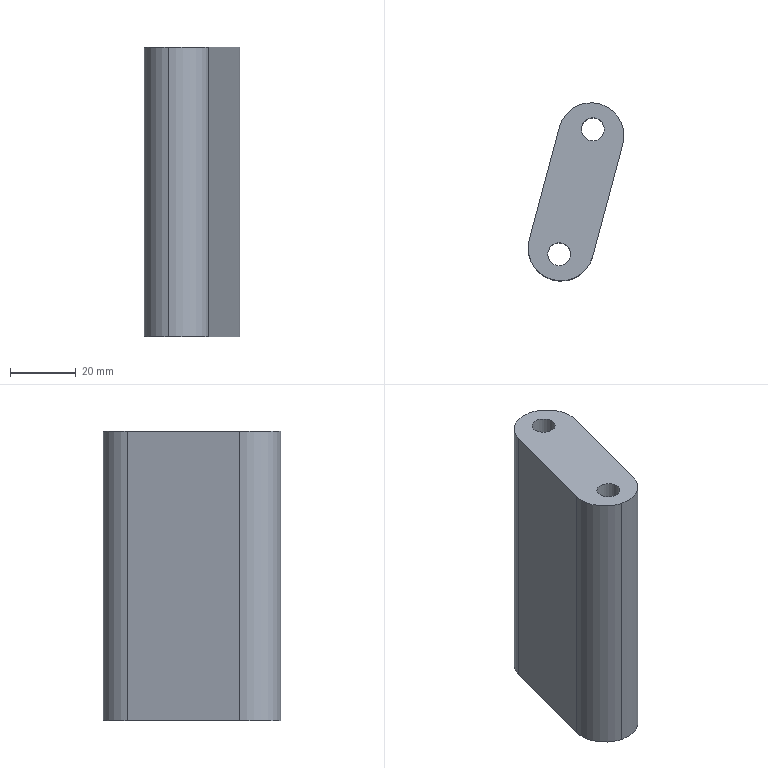Part | NX | features solid 2 | 1 solid | 14 faces | box 29.153 x 54.158 x 88 mm | volume 77441 mm3 | cylinder 8 | plane 6 | commonest cylinder face diameters 20 x4 7 x2 12 x2
STEP:
#1=CARTESIAN_POINT('',(116.417,-38.23,38.));
#2=VERTEX_POINT('',#1);
#3=CARTESIAN_POINT('',(112.917,-38.23,38.));
#4=DIRECTION('',(0.,0.,1.));
#5=DIRECTION('',(1.,0.,0.));
#6=AXIS2_PLACEMENT_3D('',#3,#4,#5);
#7=CIRCLE('',#6,3.5);
#8=EDGE_CURVE('',#2,#2,#7,.F.);
#9=ORIENTED_EDGE('',*,*,#8,.F.);
#10=EDGE_LOOP('',(#9));
#11=FACE_BOUND('',#10,.T.);
#12=CARTESIAN_POINT('',(118.917,-38.23,38.));
#13=VERTEX_POINT('',#12);
#14=CARTESIAN_POINT('',(112.917,-38.23,38.));
#15=DIRECTION('',(0.,0.,1.));
#16=DIRECTION('',(1.,0.,0.));
#17=AXIS2_PLACEMENT_3D('',#14,#15,#16);
#18=CIRCLE('',#17,6.);
#19=EDGE_CURVE('',#13,#13,#18,.F.);
#20=ORIENTED_EDGE('',*,*,#19,.T.);
#21=EDGE_LOOP('',(#20));
#22=FACE_BOUND('',#21,.T.);
#23=CARTESIAN_POINT('',(268.879,0.,38.));
#24=DIRECTION('',(0.,0.,1.));
#25=DIRECTION('',(-1.,0.,0.));
#26=AXIS2_PLACEMENT_3D('',#23,#24,#25);
#27=PLANE('',#26);
#28=ADVANCED_FACE('',(#11,#22),#27,.F.);
#29=CARTESIAN_POINT('',(116.417,-38.23,88.));
#30=VERTEX_POINT('',#29);
#31=CARTESIAN_POINT('',(112.917,-38.23,88.));
#32=DIRECTION('',(0.,0.,1.));
#33=DIRECTION('',(1.,0.,0.));
#34=AXIS2_PLACEMENT_3D('',#31,#32,#33);
#35=CIRCLE('',#34,3.5);
#36=EDGE_CURVE('',#30,#30,#35,.F.);
#37=ORIENTED_EDGE('',*,*,#36,.F.);
#38=EDGE_LOOP('',(#37));
#39=FACE_BOUND('',#38,.T.);
#40=ORIENTED_EDGE('',*,*,#8,.T.);
#41=EDGE_LOOP('',(#40));
#42=FACE_BOUND('',#41,.T.);
#43=CARTESIAN_POINT('',(112.917,-38.23,40.));
#44=DIRECTION('',(0.,0.,1.));
#45=DIRECTION('',(-0.866,0.5,0.));
#46=AXIS2_PLACEMENT_3D('',#43,#44,#45);
#47=CYLINDRICAL_SURFACE('',#46,3.5);
#48=ADVANCED_FACE('',(#39,#42),#47,.F.);
#49=ORIENTED_EDGE('',*,*,#19,.F.);
#50=EDGE_LOOP('',(#49));
#51=FACE_BOUND('',#50,.T.);
#52=CARTESIAN_POINT('',(107.721,-35.23,0.00000121));
#53=VERTEX_POINT('',#52);
#54=CARTESIAN_POINT('',(112.917,-38.23,0.00000121));
#55=DIRECTION('',(0.,0.,1.));
#56=DIRECTION('',(-0.866,0.5,0.));
#57=AXIS2_PLACEMENT_3D('',#54,#55,#56);
#58=CIRCLE('',#57,6.);
#59=EDGE_CURVE('',#53,#53,#58,.T.);
#60=ORIENTED_EDGE('',*,*,#59,.F.);
#61=EDGE_LOOP('',(#60));
#62=FACE_BOUND('',#61,.T.);
#63=CARTESIAN_POINT('',(112.917,-38.23,0.00000121));
#64=DIRECTION('',(0.,0.,1.));
#65=DIRECTION('',(-0.866,0.5,0.));
#66=AXIS2_PLACEMENT_3D('',#63,#64,#65);
#67=CYLINDRICAL_SURFACE('',#66,6.);
#68=ADVANCED_FACE('',(#51,#62),#67,.F.);
#69=CARTESIAN_POINT('',(106.229,-76.252,38.));
#70=VERTEX_POINT('',#69);
#71=CARTESIAN_POINT('',(102.729,-76.252,38.));
#72=DIRECTION('',(0.,0.,1.));
#73=DIRECTION('',(1.,0.,0.));
#74=AXIS2_PLACEMENT_3D('',#71,#72,#73);
#75=CIRCLE('',#74,3.5);
#76=EDGE_CURVE('',#70,#70,#75,.F.);
#77=ORIENTED_EDGE('',*,*,#76,.F.);
#78=EDGE_LOOP('',(#77));
#79=FACE_BOUND('',#78,.T.);
#80=CARTESIAN_POINT('',(108.729,-76.252,38.));
#81=VERTEX_POINT('',#80);
#82=CARTESIAN_POINT('',(102.729,-76.252,38.));
#83=DIRECTION('',(0.,0.,1.));
#84=DIRECTION('',(1.,0.,0.));
#85=AXIS2_PLACEMENT_3D('',#82,#83,#84);
#86=CIRCLE('',#85,6.);
#87=EDGE_CURVE('',#81,#81,#86,.F.);
#88=ORIENTED_EDGE('',*,*,#87,.T.);
#89=EDGE_LOOP('',(#88));
#90=FACE_BOUND('',#89,.T.);
#91=CARTESIAN_POINT('',(268.879,0.,38.));
#92=DIRECTION('',(0.,0.,1.));
#93=DIRECTION('',(-1.,0.,0.));
#94=AXIS2_PLACEMENT_3D('',#91,#92,#93);
#95=PLANE('',#94);
#96=ADVANCED_FACE('',(#79,#90),#95,.F.);
#97=CARTESIAN_POINT('',(112.906,-76.908,88.));
#98=VERTEX_POINT('',#97);
#99=CARTESIAN_POINT('',(122.059,-42.75,88.));
#100=VERTEX_POINT('',#99);
#101=CARTESIAN_POINT('',(142.581,33.841,88.));
#102=DIRECTION('',(0.2588,0.9659,0.));
#103=VECTOR('',#102,1000.);
#104=LINE('',#101,#103);
#105=EDGE_CURVE('',#98,#100,#104,.T.);
#106=ORIENTED_EDGE('',*,*,#105,.F.);
#107=CARTESIAN_POINT('',(112.906,-76.908,0.00000121));
#108=VERTEX_POINT('',#107);
#109=CARTESIAN_POINT('',(112.906,-76.908,-0.15));
#110=DIRECTION('',(0.,0.,-1.));
#111=VECTOR('',#110,1000.);
#112=LINE('',#109,#111);
#113=EDGE_CURVE('',#98,#108,#112,.T.);
#114=ORIENTED_EDGE('',*,*,#113,.T.);
#115=CARTESIAN_POINT('',(122.059,-42.75,0.00000121));
#116=VERTEX_POINT('',#115);
#117=CARTESIAN_POINT('',(124.199,-34.762,0.00000121));
#118=DIRECTION('',(-0.2588,-0.9659,0.));
#119=VECTOR('',#118,1000.);
#120=LINE('',#117,#119);
#121=EDGE_CURVE('',#116,#108,#120,.T.);
#122=ORIENTED_EDGE('',*,*,#121,.F.);
#123=CARTESIAN_POINT('',(122.059,-42.75,-0.15));
#124=DIRECTION('',(0.,0.,1.));
#125=VECTOR('',#124,1000.);
#126=LINE('',#123,#125);
#127=EDGE_CURVE('',#116,#100,#126,.T.);
#128=ORIENTED_EDGE('',*,*,#127,.T.);
#129=EDGE_LOOP('',(#106,#114,#122,#128));
#130=FACE_BOUND('',#129,.T.);
#131=CARTESIAN_POINT('',(117.482,-59.829,-0.15));
#132=DIRECTION('',(0.9659,-0.2588,0.));
#133=DIRECTION('',(0.2588,0.9659,0.));
#134=AXIS2_PLACEMENT_3D('',#131,#132,#133);
#135=PLANE('',#134);
#136=ADVANCED_FACE('',(#130),#135,.T.);
#137=CARTESIAN_POINT('',(93.588,-71.732,0.00000121));
#138=VERTEX_POINT('',#137);
#139=CARTESIAN_POINT('',(102.74,-37.574,0.00000121));
#140=VERTEX_POINT('',#139);
#141=CARTESIAN_POINT('',(104.881,-29.586,0.00000121));
#142=DIRECTION('',(0.2588,0.9659,0.));
#143=VECTOR('',#142,1000.);
#144=LINE('',#141,#143);
#145=EDGE_CURVE('',#138,#140,#144,.T.);
#146=ORIENTED_EDGE('',*,*,#145,.F.);
#147=CARTESIAN_POINT('',(93.588,-71.732,88.));
#148=VERTEX_POINT('',#147);
#149=CARTESIAN_POINT('',(93.588,-71.732,-0.15));
#150=DIRECTION('',(0.,0.,1.));
#151=VECTOR('',#150,1000.);
#152=LINE('',#149,#151);
#153=EDGE_CURVE('',#138,#148,#152,.T.);
#154=ORIENTED_EDGE('',*,*,#153,.T.);
#155=CARTESIAN_POINT('',(102.74,-37.574,88.));
#156=VERTEX_POINT('',#155);
#157=CARTESIAN_POINT('',(123.263,39.018,88.));
#158=DIRECTION('',(-0.2588,-0.9659,0.));
#159=VECTOR('',#158,1000.);
#160=LINE('',#157,#159);
#161=EDGE_CURVE('',#156,#148,#160,.T.);
#162=ORIENTED_EDGE('',*,*,#161,.F.);
#163=CARTESIAN_POINT('',(102.74,-37.574,-0.15));
#164=DIRECTION('',(0.,0.,-1.));
#165=VECTOR('',#164,1000.);
#166=LINE('',#163,#165);
#167=EDGE_CURVE('',#156,#140,#166,.T.);
#168=ORIENTED_EDGE('',*,*,#167,.T.);
#169=EDGE_LOOP('',(#146,#154,#162,#168));
#170=FACE_BOUND('',#169,.T.);
#171=CARTESIAN_POINT('',(98.164,-54.653,-0.15));
#172=DIRECTION('',(-0.9659,0.2588,0.));
#173=DIRECTION('',(-0.2588,-0.9659,0.));
#174=AXIS2_PLACEMENT_3D('',#171,#172,#173);
#175=PLANE('',#174);
#176=ADVANCED_FACE('',(#170),#175,.T.);
#177=CARTESIAN_POINT('',(106.229,-76.252,88.));
#178=VERTEX_POINT('',#177);
#179=CARTESIAN_POINT('',(102.729,-76.252,88.));
#180=DIRECTION('',(0.,0.,1.));
#181=DIRECTION('',(1.,0.,0.));
#182=AXIS2_PLACEMENT_3D('',#179,#180,#181);
#183=CIRCLE('',#182,3.5);
#184=EDGE_CURVE('',#178,#178,#183,.T.);
#185=ORIENTED_EDGE('',*,*,#184,.T.);
#186=EDGE_LOOP('',(#185));
#187=FACE_BOUND('',#186,.T.);
#188=ORIENTED_EDGE('',*,*,#76,.T.);
#189=EDGE_LOOP('',(#188));
#190=FACE_BOUND('',#189,.T.);
#191=CARTESIAN_POINT('',(102.729,-76.252,40.));
#192=DIRECTION('',(0.,0.,1.));
#193=DIRECTION('',(-1.,0.,0.));
#194=AXIS2_PLACEMENT_3D('',#191,#192,#193);
#195=CYLINDRICAL_SURFACE('',#194,3.5);
#196=ADVANCED_FACE('',(#187,#190),#195,.F.);
#197=ORIENTED_EDGE('',*,*,#36,.T.);
#198=EDGE_LOOP('',(#197));
#199=FACE_BOUND('',#198,.T.);
#200=ORIENTED_EDGE('',*,*,#184,.F.);
#201=EDGE_LOOP('',(#200));
#202=FACE_BOUND('',#201,.T.);
#203=ORIENTED_EDGE('',*,*,#161,.T.);
#204=CARTESIAN_POINT('',(100.659,-83.98,88.));
#205=VERTEX_POINT('',#204);
#206=CARTESIAN_POINT('',(103.247,-74.32,88.));
#207=DIRECTION('',(0.,0.,1.));
#208=DIRECTION('',(1.,0.,0.));
#209=AXIS2_PLACEMENT_3D('',#206,#207,#208);
#210=CIRCLE('',#209,10.);
#211=EDGE_CURVE('',#148,#205,#210,.T.);
#212=ORIENTED_EDGE('',*,*,#211,.T.);
#213=CARTESIAN_POINT('',(103.247,-74.32,88.));
#214=DIRECTION('',(0.,0.,1.));
#215=DIRECTION('',(1.,0.,0.));
#216=AXIS2_PLACEMENT_3D('',#213,#214,#215);
#217=CIRCLE('',#216,10.);
#218=EDGE_CURVE('',#205,#98,#217,.T.);
#219=ORIENTED_EDGE('',*,*,#218,.T.);
#220=ORIENTED_EDGE('',*,*,#105,.T.);
#221=CARTESIAN_POINT('',(114.988,-30.503,88.));
#222=VERTEX_POINT('',#221);
#223=CARTESIAN_POINT('',(112.399,-40.162,88.));
#224=DIRECTION('',(0.,0.,1.));
#225=DIRECTION('',(1.,0.,0.));
#226=AXIS2_PLACEMENT_3D('',#223,#224,#225);
#227=CIRCLE('',#226,10.);
#228=EDGE_CURVE('',#100,#222,#227,.T.);
#229=ORIENTED_EDGE('',*,*,#228,.T.);
#230=CARTESIAN_POINT('',(112.399,-40.162,88.));
#231=DIRECTION('',(0.,0.,1.));
#232=DIRECTION('',(1.,0.,0.));
#233=AXIS2_PLACEMENT_3D('',#230,#231,#232);
#234=CIRCLE('',#233,10.);
#235=EDGE_CURVE('',#222,#156,#234,.T.);
#236=ORIENTED_EDGE('',*,*,#235,.T.);
#237=EDGE_LOOP('',(#203,#212,#219,#220,#229,#236));
#238=FACE_BOUND('',#237,.T.);
#239=CARTESIAN_POINT('',(268.879,0.,88.));
#240=DIRECTION('',(0.,0.,1.));
#241=DIRECTION('',(-1.,0.,0.));
#242=AXIS2_PLACEMENT_3D('',#239,#240,#241);
#243=PLANE('',#242);
#244=ADVANCED_FACE('',(#199,#202,#238),#243,.T.);
#245=ORIENTED_EDGE('',*,*,#87,.F.);
#246=EDGE_LOOP('',(#245));
#247=FACE_BOUND('',#246,.T.);
#248=CARTESIAN_POINT('',(96.729,-76.252,0.00000121));
#249=VERTEX_POINT('',#248);
#250=CARTESIAN_POINT('',(102.729,-76.252,0.00000121));
#251=DIRECTION('',(0.,0.,-1.));
#252=DIRECTION('',(-1.,0.,0.));
#253=AXIS2_PLACEMENT_3D('',#250,#251,#252);
#254=CIRCLE('',#253,6.);
#255=EDGE_CURVE('',#249,#249,#254,.F.);
#256=ORIENTED_EDGE('',*,*,#255,.F.);
#257=EDGE_LOOP('',(#256));
#258=FACE_BOUND('',#257,.T.);
#259=CARTESIAN_POINT('',(102.729,-76.252,0.00000121));
#260=DIRECTION('',(0.,0.,1.));
#261=DIRECTION('',(-1.,0.,0.));
#262=AXIS2_PLACEMENT_3D('',#259,#260,#261);
#263=CYLINDRICAL_SURFACE('',#262,6.);
#264=ADVANCED_FACE('',(#247,#258),#263,.F.);
#265=ORIENTED_EDGE('',*,*,#59,.T.);
#266=EDGE_LOOP('',(#265));
#267=FACE_BOUND('',#266,.T.);
#268=ORIENTED_EDGE('',*,*,#255,.T.);
#269=EDGE_LOOP('',(#268));
#270=FACE_BOUND('',#269,.T.);
#271=CARTESIAN_POINT('',(114.988,-30.503,0.00000121));
#272=VERTEX_POINT('',#271);
#273=CARTESIAN_POINT('',(112.399,-40.162,0.00000121));
#274=DIRECTION('',(0.,0.,-1.));
#275=DIRECTION('',(-1.,0.,0.));
#276=AXIS2_PLACEMENT_3D('',#273,#274,#275);
#277=CIRCLE('',#276,10.);
#278=EDGE_CURVE('',#272,#116,#277,.T.);
#279=ORIENTED_EDGE('',*,*,#278,.T.);
#280=ORIENTED_EDGE('',*,*,#121,.T.);
#281=CARTESIAN_POINT('',(100.659,-83.98,0.00000121));
#282=VERTEX_POINT('',#281);
#283=CARTESIAN_POINT('',(103.247,-74.32,0.00000121));
#284=DIRECTION('',(0.,0.,-1.));
#285=DIRECTION('',(-1.,0.,0.));
#286=AXIS2_PLACEMENT_3D('',#283,#284,#285);
#287=CIRCLE('',#286,10.);
#288=EDGE_CURVE('',#108,#282,#287,.T.);
#289=ORIENTED_EDGE('',*,*,#288,.T.);
#290=CARTESIAN_POINT('',(103.247,-74.32,0.00000121));
#291=DIRECTION('',(0.,0.,-1.));
#292=DIRECTION('',(-1.,0.,0.));
#293=AXIS2_PLACEMENT_3D('',#290,#291,#292);
#294=CIRCLE('',#293,10.);
#295=EDGE_CURVE('',#282,#138,#294,.T.);
#296=ORIENTED_EDGE('',*,*,#295,.T.);
#297=ORIENTED_EDGE('',*,*,#145,.T.);
#298=CARTESIAN_POINT('',(112.399,-40.162,0.00000121));
#299=DIRECTION('',(0.,0.,-1.));
#300=DIRECTION('',(-1.,0.,0.));
#301=AXIS2_PLACEMENT_3D('',#298,#299,#300);
#302=CIRCLE('',#301,10.);
#303=EDGE_CURVE('',#140,#272,#302,.T.);
#304=ORIENTED_EDGE('',*,*,#303,.T.);
#305=EDGE_LOOP('',(#279,#280,#289,#296,#297,#304));
#306=FACE_BOUND('',#305,.T.);
#307=CARTESIAN_POINT('',(-5.534,0.,0.00000121));
#308=DIRECTION('',(0.,0.,1.));
#309=DIRECTION('',(-1.,0.,0.));
#310=AXIS2_PLACEMENT_3D('',#307,#308,#309);
#311=PLANE('',#310);
#312=ADVANCED_FACE('',(#267,#270,#306),#311,.F.);
#313=ORIENTED_EDGE('',*,*,#127,.F.);
#314=ORIENTED_EDGE('',*,*,#278,.F.);
#315=CARTESIAN_POINT('',(114.988,-30.503,-0.15));
#316=DIRECTION('',(0.,0.,1.));
#317=VECTOR('',#316,1000.);
#318=LINE('',#315,#317);
#319=EDGE_CURVE('',#222,#272,#318,.F.);
#320=ORIENTED_EDGE('',*,*,#319,.F.);
#321=ORIENTED_EDGE('',*,*,#228,.F.);
#322=EDGE_LOOP('',(#313,#314,#320,#321));
#323=FACE_BOUND('',#322,.T.);
#324=CARTESIAN_POINT('',(112.399,-40.162,-0.15));
#325=DIRECTION('',(0.,0.,1.));
#326=DIRECTION('',(-1.,0.,0.));
#327=AXIS2_PLACEMENT_3D('',#324,#325,#326);
#328=CYLINDRICAL_SURFACE('',#327,10.);
#329=ADVANCED_FACE('',(#323),#328,.T.);
#330=ORIENTED_EDGE('',*,*,#235,.F.);
#331=ORIENTED_EDGE('',*,*,#319,.T.);
#332=ORIENTED_EDGE('',*,*,#303,.F.);
#333=ORIENTED_EDGE('',*,*,#167,.F.);
#334=EDGE_LOOP('',(#330,#331,#332,#333));
#335=FACE_BOUND('',#334,.T.);
#336=CARTESIAN_POINT('',(112.399,-40.162,-0.15));
#337=DIRECTION('',(0.,0.,-1.));
#338=DIRECTION('',(1.,0.,0.));
#339=AXIS2_PLACEMENT_3D('',#336,#337,#338);
#340=CYLINDRICAL_SURFACE('',#339,10.);
#341=ADVANCED_FACE('',(#335),#340,.T.);
#342=ORIENTED_EDGE('',*,*,#113,.F.);
#343=ORIENTED_EDGE('',*,*,#218,.F.);
#344=CARTESIAN_POINT('',(100.659,-83.98,-0.15));
#345=DIRECTION('',(0.,0.,-1.));
#346=VECTOR('',#345,1000.);
#347=LINE('',#344,#346);
#348=EDGE_CURVE('',#282,#205,#347,.F.);
#349=ORIENTED_EDGE('',*,*,#348,.F.);
#350=ORIENTED_EDGE('',*,*,#288,.F.);
#351=EDGE_LOOP('',(#342,#343,#349,#350));
#352=FACE_BOUND('',#351,.T.);
#353=CARTESIAN_POINT('',(103.247,-74.32,-0.15));
#354=DIRECTION('',(0.,0.,-1.));
#355=DIRECTION('',(1.,0.,0.));
#356=AXIS2_PLACEMENT_3D('',#353,#354,#355);
#357=CYLINDRICAL_SURFACE('',#356,10.);
#358=ADVANCED_FACE('',(#352),#357,.T.);
#359=ORIENTED_EDGE('',*,*,#295,.F.);
#360=ORIENTED_EDGE('',*,*,#348,.T.);
#361=ORIENTED_EDGE('',*,*,#211,.F.);
#362=ORIENTED_EDGE('',*,*,#153,.F.);
#363=EDGE_LOOP('',(#359,#360,#361,#362));
#364=FACE_BOUND('',#363,.T.);
#365=CARTESIAN_POINT('',(103.247,-74.32,-0.15));
#366=DIRECTION('',(0.,0.,1.));
#367=DIRECTION('',(-1.,0.,0.));
#368=AXIS2_PLACEMENT_3D('',#365,#366,#367);
#369=CYLINDRICAL_SURFACE('',#368,10.);
#370=ADVANCED_FACE('',(#364),#369,.T.);
#371=CLOSED_SHELL('',(#28,#48,#68,#96,#136,#176,#196,#244,#264,#312,#329,#341,#358,#370));
#372=MANIFOLD_SOLID_BREP('',#371);
#373=(LENGTH_UNIT()NAMED_UNIT(*)SI_UNIT(.MILLI.,.METRE.));
#374=UNCERTAINTY_MEASURE_WITH_UNIT(LENGTH_MEASURE(0.00001),#373,'','');
#375=(NAMED_UNIT(*)PLANE_ANGLE_UNIT()SI_UNIT($,.RADIAN.));
#376=(NAMED_UNIT(*)SI_UNIT($,.STERADIAN.)SOLID_ANGLE_UNIT());
#377=(GEOMETRIC_REPRESENTATION_CONTEXT(3)GLOBAL_UNCERTAINTY_ASSIGNED_CONTEXT((#374))GLOBAL_UNIT_ASSIGNED_CONTEXT((#373,#375,#376))REPRESENTATION_CONTEXT('',''));
#378=ADVANCED_BREP_SHAPE_REPRESENTATION('',(#372),#377);